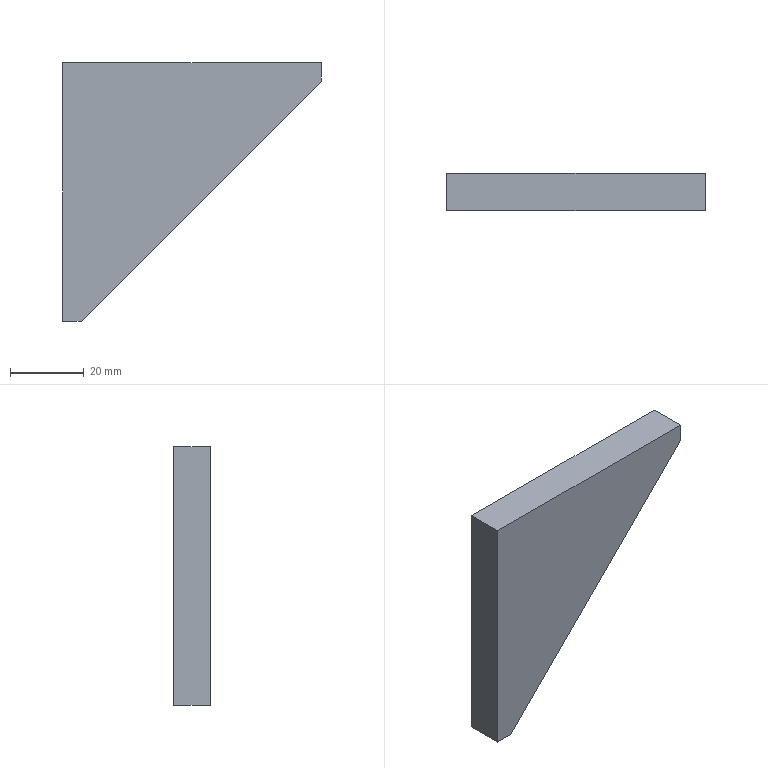Part | STEP file | Positioning_id1830_x_t | 1 solid | 7 faces | box 70 x 10 x 70 mm | volume 27875 mm3 | plane 7
STEP:
#1=CARTESIAN_POINT('',(0.,0.,0.));
#2=DIRECTION('',(0.,0.,1.));
#3=DIRECTION('',(1.,0.,0.));
#4=AXIS2_PLACEMENT_3D('',#1,#2,#3);
#5=CARTESIAN_POINT('',(-928.002,386.,126.5));
#6=VERTEX_POINT('',#5);
#7=CARTESIAN_POINT('',(-993.002,386.,61.5));
#8=VERTEX_POINT('',#7);
#9=CARTESIAN_POINT('',(-928.002,386.,126.5));
#10=DIRECTION('',(-0.7071,0.,-0.7071));
#11=VECTOR('',#10,1.);
#12=LINE('',#9,#11);
#13=CARTESIAN_POINT('',(-993.002,391.,61.5));
#14=DIRECTION('',(-0.7071,0.,0.7071));
#15=DIRECTION('',(-0.7071,0.,-0.7071));
#16=AXIS2_PLACEMENT_3D('',#13,#14,#15);
#17=PLANE('',#16);
#18=CARTESIAN_POINT('',(-91.924,5.));
#19=DIRECTION('',(1.,0.));
#20=VECTOR('',#19,1.);
#21=LINE('',#18,#20);
#22=(GEOMETRIC_REPRESENTATION_CONTEXT(2)PARAMETRIC_REPRESENTATION_CONTEXT()REPRESENTATION_CONTEXT('',''));
#23=DEFINITIONAL_REPRESENTATION('',(#21),#22);
#24=PCURVE('',#17,#23);
#25=CARTESIAN_POINT('',(-948.002,386.,91.5));
#26=DIRECTION('',(0.,-1.,0.));
#27=DIRECTION('',(-1.,0.,0.));
#28=AXIS2_PLACEMENT_3D('',#25,#26,#27);
#29=PLANE('',#28);
#30=CARTESIAN_POINT('',(-20.,-35.));
#31=DIRECTION('',(0.7071,0.7071));
#32=VECTOR('',#31,1.);
#33=LINE('',#30,#32);
#34=(GEOMETRIC_REPRESENTATION_CONTEXT(2)PARAMETRIC_REPRESENTATION_CONTEXT()REPRESENTATION_CONTEXT('',''));
#35=DEFINITIONAL_REPRESENTATION('',(#33),#34);
#36=PCURVE('',#29,#35);
#37=SURFACE_CURVE('',#12,(#24,#36),.PCURVE_S1.);
#38=EDGE_CURVE('',#6,#8,#37,.T.);
#39=ORIENTED_EDGE('',*,*,#38,.T.);
#40=CARTESIAN_POINT('',(-993.002,396.,61.5));
#41=VERTEX_POINT('',#40);
#42=CARTESIAN_POINT('',(-993.002,386.,61.5));
#43=DIRECTION('',(0.,1.,0.));
#44=VECTOR('',#43,1.);
#45=LINE('',#42,#44);
#46=CARTESIAN_POINT('',(0.,5.));
#47=DIRECTION('',(0.,-1.));
#48=VECTOR('',#47,1.);
#49=LINE('',#46,#48);
#50=(GEOMETRIC_REPRESENTATION_CONTEXT(2)PARAMETRIC_REPRESENTATION_CONTEXT()REPRESENTATION_CONTEXT('',''));
#51=DEFINITIONAL_REPRESENTATION('',(#49),#50);
#52=PCURVE('',#17,#51);
#53=CARTESIAN_POINT('',(-948.002,391.,61.5));
#54=DIRECTION('',(0.,0.,-1.));
#55=DIRECTION('',(0.,1.,0.));
#56=AXIS2_PLACEMENT_3D('',#53,#54,#55);
#57=PLANE('',#56);
#58=CARTESIAN_POINT('',(-5.,-45.));
#59=DIRECTION('',(1.,0.));
#60=VECTOR('',#59,1.);
#61=LINE('',#58,#60);
#62=(GEOMETRIC_REPRESENTATION_CONTEXT(2)PARAMETRIC_REPRESENTATION_CONTEXT()REPRESENTATION_CONTEXT('',''));
#63=DEFINITIONAL_REPRESENTATION('',(#61),#62);
#64=PCURVE('',#57,#63);
#65=SURFACE_CURVE('',#45,(#52,#64),.PCURVE_S1.);
#66=EDGE_CURVE('',#8,#41,#65,.T.);
#67=ORIENTED_EDGE('',*,*,#66,.T.);
#68=CARTESIAN_POINT('',(-928.002,396.,126.5));
#69=VERTEX_POINT('',#68);
#70=CARTESIAN_POINT('',(-993.002,396.,61.5));
#71=DIRECTION('',(0.7071,0.,0.7071));
#72=VECTOR('',#71,1.);
#73=LINE('',#70,#72);
#74=CARTESIAN_POINT('',(0.,-5.));
#75=DIRECTION('',(-1.,0.));
#76=VECTOR('',#75,1.);
#77=LINE('',#74,#76);
#78=(GEOMETRIC_REPRESENTATION_CONTEXT(2)PARAMETRIC_REPRESENTATION_CONTEXT()REPRESENTATION_CONTEXT('',''));
#79=DEFINITIONAL_REPRESENTATION('',(#77),#78);
#80=PCURVE('',#17,#79);
#81=CARTESIAN_POINT('',(-948.002,396.,91.5));
#82=DIRECTION('',(0.,1.,0.));
#83=DIRECTION('',(1.,0.,0.));
#84=AXIS2_PLACEMENT_3D('',#81,#82,#83);
#85=PLANE('',#84);
#86=CARTESIAN_POINT('',(-45.,30.));
#87=DIRECTION('',(0.7071,-0.7071));
#88=VECTOR('',#87,1.);
#89=LINE('',#86,#88);
#90=(GEOMETRIC_REPRESENTATION_CONTEXT(2)PARAMETRIC_REPRESENTATION_CONTEXT()REPRESENTATION_CONTEXT('',''));
#91=DEFINITIONAL_REPRESENTATION('',(#89),#90);
#92=PCURVE('',#85,#91);
#93=SURFACE_CURVE('',#73,(#80,#92),.PCURVE_S1.);
#94=EDGE_CURVE('',#41,#69,#93,.T.);
#95=ORIENTED_EDGE('',*,*,#94,.T.);
#96=CARTESIAN_POINT('',(-928.002,396.,126.5));
#97=DIRECTION('',(0.,-1.,0.));
#98=VECTOR('',#97,1.);
#99=LINE('',#96,#98);
#100=CARTESIAN_POINT('',(-91.924,-5.));
#101=DIRECTION('',(0.,1.));
#102=VECTOR('',#101,1.);
#103=LINE('',#100,#102);
#104=(GEOMETRIC_REPRESENTATION_CONTEXT(2)PARAMETRIC_REPRESENTATION_CONTEXT()REPRESENTATION_CONTEXT('',''));
#105=DEFINITIONAL_REPRESENTATION('',(#103),#104);
#106=PCURVE('',#17,#105);
#107=CARTESIAN_POINT('',(-928.002,391.,91.5));
#108=DIRECTION('',(1.,0.,0.));
#109=DIRECTION('',(0.,-1.,0.));
#110=AXIS2_PLACEMENT_3D('',#107,#108,#109);
#111=PLANE('',#110);
#112=CARTESIAN_POINT('',(-5.,-35.));
#113=DIRECTION('',(1.,0.));
#114=VECTOR('',#113,1.);
#115=LINE('',#112,#114);
#116=(GEOMETRIC_REPRESENTATION_CONTEXT(2)PARAMETRIC_REPRESENTATION_CONTEXT()REPRESENTATION_CONTEXT('',''));
#117=DEFINITIONAL_REPRESENTATION('',(#115),#116);
#118=PCURVE('',#111,#117);
#119=SURFACE_CURVE('',#99,(#106,#118),.PCURVE_S1.);
#120=EDGE_CURVE('',#69,#6,#119,.T.);
#121=ORIENTED_EDGE('',*,*,#120,.T.);
#122=EDGE_LOOP('',(#39,#67,#95,#121));
#123=FACE_BOUND('',#122,.T.);
#124=ADVANCED_FACE('',(#123),#17,.F.);
#125=CARTESIAN_POINT('',(-928.002,396.,131.5));
#126=VERTEX_POINT('',#125);
#127=CARTESIAN_POINT('',(-928.002,396.,131.5));
#128=DIRECTION('',(0.,0.,-1.));
#129=VECTOR('',#128,1.);
#130=LINE('',#127,#129);
#131=CARTESIAN_POINT('',(-5.,-40.));
#132=DIRECTION('',(0.,1.));
#133=VECTOR('',#132,1.);
#134=LINE('',#131,#133);
#135=(GEOMETRIC_REPRESENTATION_CONTEXT(2)PARAMETRIC_REPRESENTATION_CONTEXT()REPRESENTATION_CONTEXT('',''));
#136=DEFINITIONAL_REPRESENTATION('',(#134),#135);
#137=PCURVE('',#111,#136);
#138=CARTESIAN_POINT('',(20.,-40.));
#139=DIRECTION('',(0.,1.));
#140=VECTOR('',#139,1.);
#141=LINE('',#138,#140);
#142=(GEOMETRIC_REPRESENTATION_CONTEXT(2)PARAMETRIC_REPRESENTATION_CONTEXT()REPRESENTATION_CONTEXT('',''));
#143=DEFINITIONAL_REPRESENTATION('',(#141),#142);
#144=PCURVE('',#85,#143);
#145=SURFACE_CURVE('',#130,(#137,#144),.PCURVE_S1.);
#146=EDGE_CURVE('',#126,#69,#145,.T.);
#147=ORIENTED_EDGE('',*,*,#146,.F.);
#148=CARTESIAN_POINT('',(-928.002,386.,131.5));
#149=VERTEX_POINT('',#148);
#150=CARTESIAN_POINT('',(-928.002,396.,131.5));
#151=DIRECTION('',(0.,-1.,0.));
#152=VECTOR('',#151,1.);
#153=LINE('',#150,#152);
#154=CARTESIAN_POINT('',(-5.,-40.));
#155=DIRECTION('',(1.,0.));
#156=VECTOR('',#155,1.);
#157=LINE('',#154,#156);
#158=(GEOMETRIC_REPRESENTATION_CONTEXT(2)PARAMETRIC_REPRESENTATION_CONTEXT()REPRESENTATION_CONTEXT('',''));
#159=DEFINITIONAL_REPRESENTATION('',(#157),#158);
#160=PCURVE('',#111,#159);
#161=CARTESIAN_POINT('',(-948.002,391.,131.5));
#162=DIRECTION('',(0.,0.,1.));
#163=DIRECTION('',(0.,-1.,0.));
#164=AXIS2_PLACEMENT_3D('',#161,#162,#163);
#165=PLANE('',#164);
#166=CARTESIAN_POINT('',(-5.,20.));
#167=DIRECTION('',(1.,0.));
#168=VECTOR('',#167,1.);
#169=LINE('',#166,#168);
#170=(GEOMETRIC_REPRESENTATION_CONTEXT(2)PARAMETRIC_REPRESENTATION_CONTEXT()REPRESENTATION_CONTEXT('',''));
#171=DEFINITIONAL_REPRESENTATION('',(#169),#170);
#172=PCURVE('',#165,#171);
#173=SURFACE_CURVE('',#153,(#160,#172),.PCURVE_S1.);
#174=EDGE_CURVE('',#126,#149,#173,.T.);
#175=ORIENTED_EDGE('',*,*,#174,.T.);
#176=CARTESIAN_POINT('',(-928.002,386.,126.5));
#177=DIRECTION('',(0.,0.,1.));
#178=VECTOR('',#177,1.);
#179=LINE('',#176,#178);
#180=CARTESIAN_POINT('',(5.,-35.));
#181=DIRECTION('',(0.,-1.));
#182=VECTOR('',#181,1.);
#183=LINE('',#180,#182);
#184=(GEOMETRIC_REPRESENTATION_CONTEXT(2)PARAMETRIC_REPRESENTATION_CONTEXT()REPRESENTATION_CONTEXT('',''));
#185=DEFINITIONAL_REPRESENTATION('',(#183),#184);
#186=PCURVE('',#111,#185);
#187=CARTESIAN_POINT('',(-20.,-35.));
#188=DIRECTION('',(0.,-1.));
#189=VECTOR('',#188,1.);
#190=LINE('',#187,#189);
#191=(GEOMETRIC_REPRESENTATION_CONTEXT(2)PARAMETRIC_REPRESENTATION_CONTEXT()REPRESENTATION_CONTEXT('',''));
#192=DEFINITIONAL_REPRESENTATION('',(#190),#191);
#193=PCURVE('',#29,#192);
#194=SURFACE_CURVE('',#179,(#186,#193),.PCURVE_S1.);
#195=EDGE_CURVE('',#6,#149,#194,.T.);
#196=ORIENTED_EDGE('',*,*,#195,.F.);
#197=ORIENTED_EDGE('',*,*,#120,.F.);
#198=EDGE_LOOP('',(#147,#175,#196,#197));
#199=FACE_BOUND('',#198,.T.);
#200=ADVANCED_FACE('',(#199),#111,.T.);
#201=CARTESIAN_POINT('',(-998.002,396.,61.5));
#202=VERTEX_POINT('',#201);
#203=CARTESIAN_POINT('',(-993.002,396.,61.5));
#204=DIRECTION('',(-1.,0.,0.));
#205=VECTOR('',#204,1.);
#206=LINE('',#203,#205);
#207=CARTESIAN_POINT('',(-45.,30.));
#208=DIRECTION('',(-1.,0.));
#209=VECTOR('',#208,1.);
#210=LINE('',#207,#209);
#211=(GEOMETRIC_REPRESENTATION_CONTEXT(2)PARAMETRIC_REPRESENTATION_CONTEXT()REPRESENTATION_CONTEXT('',''));
#212=DEFINITIONAL_REPRESENTATION('',(#210),#211);
#213=PCURVE('',#85,#212);
#214=CARTESIAN_POINT('',(5.,-45.));
#215=DIRECTION('',(0.,-1.));
#216=VECTOR('',#215,1.);
#217=LINE('',#214,#216);
#218=(GEOMETRIC_REPRESENTATION_CONTEXT(2)PARAMETRIC_REPRESENTATION_CONTEXT()REPRESENTATION_CONTEXT('',''));
#219=DEFINITIONAL_REPRESENTATION('',(#217),#218);
#220=PCURVE('',#57,#219);
#221=SURFACE_CURVE('',#206,(#213,#220),.PCURVE_S1.);
#222=EDGE_CURVE('',#41,#202,#221,.T.);
#223=ORIENTED_EDGE('',*,*,#222,.T.);
#224=CARTESIAN_POINT('',(-998.002,396.,131.5));
#225=VERTEX_POINT('',#224);
#226=CARTESIAN_POINT('',(-998.002,396.,61.5));
#227=DIRECTION('',(0.,0.,1.));
#228=VECTOR('',#227,1.);
#229=LINE('',#226,#228);
#230=CARTESIAN_POINT('',(-50.,30.));
#231=DIRECTION('',(0.,-1.));
#232=VECTOR('',#231,1.);
#233=LINE('',#230,#232);
#234=(GEOMETRIC_REPRESENTATION_CONTEXT(2)PARAMETRIC_REPRESENTATION_CONTEXT()REPRESENTATION_CONTEXT('',''));
#235=DEFINITIONAL_REPRESENTATION('',(#233),#234);
#236=PCURVE('',#85,#235);
#237=CARTESIAN_POINT('',(-998.002,391.,91.5));
#238=DIRECTION('',(-1.,0.,0.));
#239=DIRECTION('',(0.,1.,0.));
#240=AXIS2_PLACEMENT_3D('',#237,#238,#239);
#241=PLANE('',#240);
#242=CARTESIAN_POINT('',(5.,30.));
#243=DIRECTION('',(0.,-1.));
#244=VECTOR('',#243,1.);
#245=LINE('',#242,#244);
#246=(GEOMETRIC_REPRESENTATION_CONTEXT(2)PARAMETRIC_REPRESENTATION_CONTEXT()REPRESENTATION_CONTEXT('',''));
#247=DEFINITIONAL_REPRESENTATION('',(#245),#246);
#248=PCURVE('',#241,#247);
#249=SURFACE_CURVE('',#229,(#236,#248),.PCURVE_S1.);
#250=EDGE_CURVE('',#202,#225,#249,.T.);
#251=ORIENTED_EDGE('',*,*,#250,.T.);
#252=CARTESIAN_POINT('',(-998.002,396.,131.5));
#253=DIRECTION('',(1.,0.,0.));
#254=VECTOR('',#253,1.);
#255=LINE('',#252,#254);
#256=CARTESIAN_POINT('',(-50.,-40.));
#257=DIRECTION('',(1.,0.));
#258=VECTOR('',#257,1.);
#259=LINE('',#256,#258);
#260=(GEOMETRIC_REPRESENTATION_CONTEXT(2)PARAMETRIC_REPRESENTATION_CONTEXT()REPRESENTATION_CONTEXT('',''));
#261=DEFINITIONAL_REPRESENTATION('',(#259),#260);
#262=PCURVE('',#85,#261);
#263=CARTESIAN_POINT('',(-5.,-50.));
#264=DIRECTION('',(0.,1.));
#265=VECTOR('',#264,1.);
#266=LINE('',#263,#265);
#267=(GEOMETRIC_REPRESENTATION_CONTEXT(2)PARAMETRIC_REPRESENTATION_CONTEXT()REPRESENTATION_CONTEXT('',''));
#268=DEFINITIONAL_REPRESENTATION('',(#266),#267);
#269=PCURVE('',#165,#268);
#270=SURFACE_CURVE('',#255,(#262,#269),.PCURVE_S1.);
#271=EDGE_CURVE('',#225,#126,#270,.T.);
#272=ORIENTED_EDGE('',*,*,#271,.T.);
#273=ORIENTED_EDGE('',*,*,#146,.T.);
#274=ORIENTED_EDGE('',*,*,#94,.F.);
#275=EDGE_LOOP('',(#223,#251,#272,#273,#274));
#276=FACE_BOUND('',#275,.T.);
#277=ADVANCED_FACE('',(#276),#85,.T.);
#278=CARTESIAN_POINT('',(-998.002,386.,61.5));
#279=VERTEX_POINT('',#278);
#280=CARTESIAN_POINT('',(-998.002,386.,61.5));
#281=DIRECTION('',(1.,0.,0.));
#282=VECTOR('',#281,1.);
#283=LINE('',#280,#282);
#284=CARTESIAN_POINT('',(-5.,-50.));
#285=DIRECTION('',(0.,1.));
#286=VECTOR('',#285,1.);
#287=LINE('',#284,#286);
#288=(GEOMETRIC_REPRESENTATION_CONTEXT(2)PARAMETRIC_REPRESENTATION_CONTEXT()REPRESENTATION_CONTEXT('',''));
#289=DEFINITIONAL_REPRESENTATION('',(#287),#288);
#290=PCURVE('',#57,#289);
#291=CARTESIAN_POINT('',(50.,30.));
#292=DIRECTION('',(-1.,0.));
#293=VECTOR('',#292,1.);
#294=LINE('',#291,#293);
#295=(GEOMETRIC_REPRESENTATION_CONTEXT(2)PARAMETRIC_REPRESENTATION_CONTEXT()REPRESENTATION_CONTEXT('',''));
#296=DEFINITIONAL_REPRESENTATION('',(#294),#295);
#297=PCURVE('',#29,#296);
#298=SURFACE_CURVE('',#283,(#290,#297),.PCURVE_S1.);
#299=EDGE_CURVE('',#279,#8,#298,.T.);
#300=ORIENTED_EDGE('',*,*,#299,.F.);
#301=CARTESIAN_POINT('',(-998.002,396.,61.5));
#302=DIRECTION('',(0.,-1.,0.));
#303=VECTOR('',#302,1.);
#304=LINE('',#301,#303);
#305=CARTESIAN_POINT('',(5.,-50.));
#306=DIRECTION('',(-1.,0.));
#307=VECTOR('',#306,1.);
#308=LINE('',#305,#307);
#309=(GEOMETRIC_REPRESENTATION_CONTEXT(2)PARAMETRIC_REPRESENTATION_CONTEXT()REPRESENTATION_CONTEXT('',''));
#310=DEFINITIONAL_REPRESENTATION('',(#308),#309);
#311=PCURVE('',#57,#310);
#312=CARTESIAN_POINT('',(5.,30.));
#313=DIRECTION('',(-1.,0.));
#314=VECTOR('',#313,1.);
#315=LINE('',#312,#314);
#316=(GEOMETRIC_REPRESENTATION_CONTEXT(2)PARAMETRIC_REPRESENTATION_CONTEXT()REPRESENTATION_CONTEXT('',''));
#317=DEFINITIONAL_REPRESENTATION('',(#315),#316);
#318=PCURVE('',#241,#317);
#319=SURFACE_CURVE('',#304,(#311,#318),.PCURVE_S1.);
#320=EDGE_CURVE('',#202,#279,#319,.T.);
#321=ORIENTED_EDGE('',*,*,#320,.F.);
#322=ORIENTED_EDGE('',*,*,#222,.F.);
#323=ORIENTED_EDGE('',*,*,#66,.F.);
#324=EDGE_LOOP('',(#300,#321,#322,#323));
#325=FACE_BOUND('',#324,.T.);
#326=ADVANCED_FACE('',(#325),#57,.T.);
#327=CARTESIAN_POINT('',(-998.002,386.,131.5));
#328=VERTEX_POINT('',#327);
#329=CARTESIAN_POINT('',(-998.002,396.,131.5));
#330=DIRECTION('',(0.,-1.,0.));
#331=VECTOR('',#330,1.);
#332=LINE('',#329,#331);
#333=CARTESIAN_POINT('',(5.,-40.));
#334=DIRECTION('',(-1.,0.));
#335=VECTOR('',#334,1.);
#336=LINE('',#333,#335);
#337=(GEOMETRIC_REPRESENTATION_CONTEXT(2)PARAMETRIC_REPRESENTATION_CONTEXT()REPRESENTATION_CONTEXT('',''));
#338=DEFINITIONAL_REPRESENTATION('',(#336),#337);
#339=PCURVE('',#241,#338);
#340=CARTESIAN_POINT('',(-5.,-50.));
#341=DIRECTION('',(1.,0.));
#342=VECTOR('',#341,1.);
#343=LINE('',#340,#342);
#344=(GEOMETRIC_REPRESENTATION_CONTEXT(2)PARAMETRIC_REPRESENTATION_CONTEXT()REPRESENTATION_CONTEXT('',''));
#345=DEFINITIONAL_REPRESENTATION('',(#343),#344);
#346=PCURVE('',#165,#345);
#347=SURFACE_CURVE('',#332,(#339,#346),.PCURVE_S1.);
#348=EDGE_CURVE('',#225,#328,#347,.T.);
#349=ORIENTED_EDGE('',*,*,#348,.F.);
#350=ORIENTED_EDGE('',*,*,#250,.F.);
#351=ORIENTED_EDGE('',*,*,#320,.T.);
#352=CARTESIAN_POINT('',(-998.002,386.,131.5));
#353=DIRECTION('',(0.,0.,-1.));
#354=VECTOR('',#353,1.);
#355=LINE('',#352,#354);
#356=CARTESIAN_POINT('',(-5.,-40.));
#357=DIRECTION('',(0.,1.));
#358=VECTOR('',#357,1.);
#359=LINE('',#356,#358);
#360=(GEOMETRIC_REPRESENTATION_CONTEXT(2)PARAMETRIC_REPRESENTATION_CONTEXT()REPRESENTATION_CONTEXT('',''));
#361=DEFINITIONAL_REPRESENTATION('',(#359),#360);
#362=PCURVE('',#241,#361);
#363=CARTESIAN_POINT('',(50.,-40.));
#364=DIRECTION('',(0.,1.));
#365=VECTOR('',#364,1.);
#366=LINE('',#363,#365);
#367=(GEOMETRIC_REPRESENTATION_CONTEXT(2)PARAMETRIC_REPRESENTATION_CONTEXT()REPRESENTATION_CONTEXT('',''));
#368=DEFINITIONAL_REPRESENTATION('',(#366),#367);
#369=PCURVE('',#29,#368);
#370=SURFACE_CURVE('',#355,(#362,#369),.PCURVE_S1.);
#371=EDGE_CURVE('',#328,#279,#370,.T.);
#372=ORIENTED_EDGE('',*,*,#371,.F.);
#373=EDGE_LOOP('',(#349,#350,#351,#372));
#374=FACE_BOUND('',#373,.T.);
#375=ADVANCED_FACE('',(#374),#241,.T.);
#376=ORIENTED_EDGE('',*,*,#174,.F.);
#377=ORIENTED_EDGE('',*,*,#271,.F.);
#378=ORIENTED_EDGE('',*,*,#348,.T.);
#379=CARTESIAN_POINT('',(-928.002,386.,131.5));
#380=DIRECTION('',(-1.,0.,0.));
#381=VECTOR('',#380,1.);
#382=LINE('',#379,#381);
#383=CARTESIAN_POINT('',(5.,20.));
#384=DIRECTION('',(0.,-1.));
#385=VECTOR('',#384,1.);
#386=LINE('',#383,#385);
#387=(GEOMETRIC_REPRESENTATION_CONTEXT(2)PARAMETRIC_REPRESENTATION_CONTEXT()REPRESENTATION_CONTEXT('',''));
#388=DEFINITIONAL_REPRESENTATION('',(#386),#387);
#389=PCURVE('',#165,#388);
#390=CARTESIAN_POINT('',(-20.,-40.));
#391=DIRECTION('',(1.,0.));
#392=VECTOR('',#391,1.);
#393=LINE('',#390,#392);
#394=(GEOMETRIC_REPRESENTATION_CONTEXT(2)PARAMETRIC_REPRESENTATION_CONTEXT()REPRESENTATION_CONTEXT('',''));
#395=DEFINITIONAL_REPRESENTATION('',(#393),#394);
#396=PCURVE('',#29,#395);
#397=SURFACE_CURVE('',#382,(#389,#396),.PCURVE_S1.);
#398=EDGE_CURVE('',#149,#328,#397,.T.);
#399=ORIENTED_EDGE('',*,*,#398,.F.);
#400=EDGE_LOOP('',(#376,#377,#378,#399));
#401=FACE_BOUND('',#400,.T.);
#402=ADVANCED_FACE('',(#401),#165,.T.);
#403=ORIENTED_EDGE('',*,*,#195,.T.);
#404=ORIENTED_EDGE('',*,*,#398,.T.);
#405=ORIENTED_EDGE('',*,*,#371,.T.);
#406=ORIENTED_EDGE('',*,*,#299,.T.);
#407=ORIENTED_EDGE('',*,*,#38,.F.);
#408=EDGE_LOOP('',(#403,#404,#405,#406,#407));
#409=FACE_BOUND('',#408,.T.);
#410=ADVANCED_FACE('',(#409),#29,.T.);
#411=CLOSED_SHELL('',(#124,#200,#277,#326,#375,#402,#410));
#412=MANIFOLD_SOLID_BREP('',#411);
#413=(LENGTH_UNIT()NAMED_UNIT(*)SI_UNIT(.MILLI.,.METRE.));
#414=UNCERTAINTY_MEASURE_WITH_UNIT(LENGTH_MEASURE(0.0000001),#413,'','');
#415=(NAMED_UNIT(*)PLANE_ANGLE_UNIT()SI_UNIT($,.RADIAN.));
#416=(NAMED_UNIT(*)SI_UNIT($,.STERADIAN.)SOLID_ANGLE_UNIT());
#417=(GEOMETRIC_REPRESENTATION_CONTEXT(3)GLOBAL_UNCERTAINTY_ASSIGNED_CONTEXT((#414))GLOBAL_UNIT_ASSIGNED_CONTEXT((#413,#415,#416))REPRESENTATION_CONTEXT('',''));
#418=ADVANCED_BREP_SHAPE_REPRESENTATION('',(#4,#412),#417);